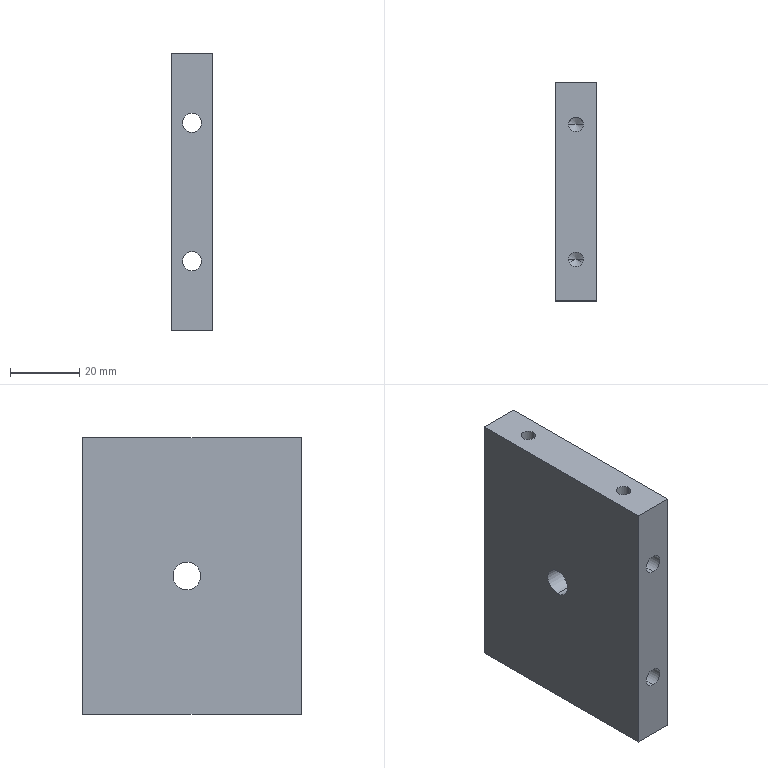Part | SolidWorks | features HoleWzd 7, Extrusion 1 | 1 solid | 52 faces | box 12 x 63 x 80 mm | volume 50248 mm3 | cylinder 28 | cone 16 | plane 8 | commonest cylinder face diameters 4.2 x18 5.5 x4 9.9 x4 8 x2